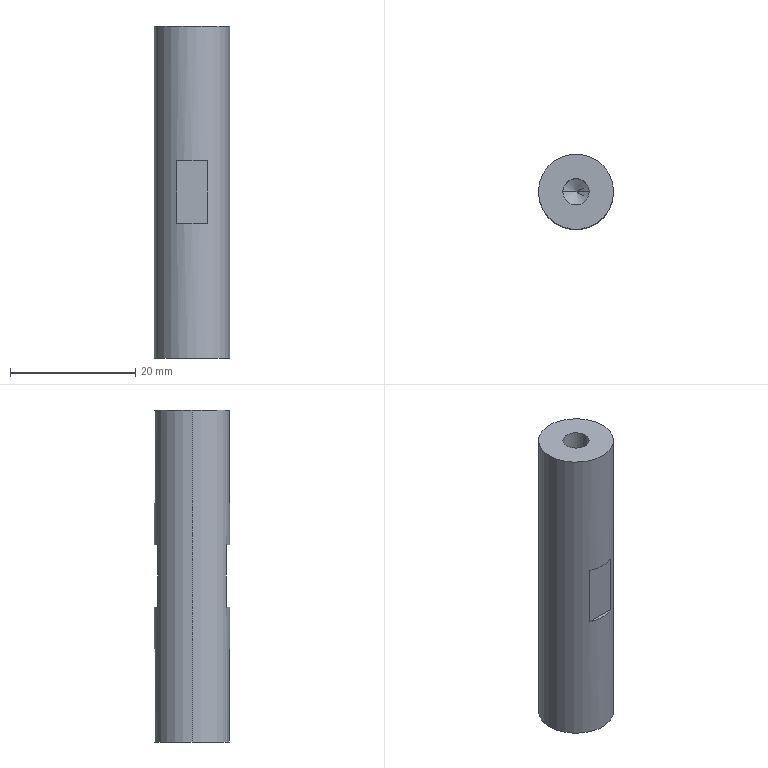Part | STEP file | 11-FG-E03911 | 1 solid | 18 faces | box 12 x 12 x 53 mm | volume 5607 mm3 | plane 8 | cylinder 6 | cone 4 | commonest cylinder face diameters 4.2 x4 12 x2
STEP:
#1=CARTESIAN_POINT('',(2.1,0.,12.4));
#2=VERTEX_POINT('',#1);
#3=CARTESIAN_POINT('',(-2.1,0.,12.4));
#4=VERTEX_POINT('',#3);
#5=CARTESIAN_POINT('',(0.,0.,12.4));
#6=DIRECTION('',(0.,0.,-1.));
#7=DIRECTION('',(-1.,0.,0.));
#8=AXIS2_PLACEMENT_3D('',#5,#6,#7);
#9=CIRCLE('',#8,2.1);
#10=EDGE_CURVE('',#2,#4,#9,.T.);
#11=ORIENTED_EDGE('',*,*,#10,.F.);
#12=CARTESIAN_POINT('',(2.1,0.,0.));
#13=VERTEX_POINT('',#12);
#14=CARTESIAN_POINT('',(2.1,0.,0.));
#15=DIRECTION('',(0.,0.,-1.));
#16=VECTOR('',#15,1000.);
#17=LINE('',#14,#16);
#18=EDGE_CURVE('',#2,#13,#17,.T.);
#19=ORIENTED_EDGE('',*,*,#18,.T.);
#20=CARTESIAN_POINT('',(-2.1,0.,0.));
#21=VERTEX_POINT('',#20);
#22=CARTESIAN_POINT('',(0.,0.,0.));
#23=DIRECTION('',(0.,0.,-1.));
#24=DIRECTION('',(-1.,0.,0.));
#25=AXIS2_PLACEMENT_3D('',#22,#23,#24);
#26=CIRCLE('',#25,2.1);
#27=EDGE_CURVE('',#13,#21,#26,.T.);
#28=ORIENTED_EDGE('',*,*,#27,.T.);
#29=CARTESIAN_POINT('',(-2.1,0.,0.));
#30=DIRECTION('',(0.,0.,-1.));
#31=VECTOR('',#30,1000.);
#32=LINE('',#29,#31);
#33=EDGE_CURVE('',#4,#21,#32,.T.);
#34=ORIENTED_EDGE('',*,*,#33,.F.);
#35=EDGE_LOOP('',(#11,#19,#28,#34));
#36=FACE_OUTER_BOUND('',#35,.T.);
#37=CARTESIAN_POINT('',(0.,0.,0.));
#38=DIRECTION('',(0.,0.,-1.));
#39=DIRECTION('',(-1.,0.,0.));
#40=AXIS2_PLACEMENT_3D('',#37,#38,#39);
#41=CYLINDRICAL_SURFACE('',#40,2.1);
#42=ADVANCED_FACE('',(#36),#41,.F.);
#43=CARTESIAN_POINT('',(0.,0.,13.662));
#44=VERTEX_POINT('',#43);
#45=CARTESIAN_POINT('',(-2.1,0.,12.4));
#46=DIRECTION('',(-0.8572,0.,-0.515));
#47=VECTOR('',#46,1000.);
#48=LINE('',#45,#47);
#49=EDGE_CURVE('',#44,#4,#48,.T.);
#50=ORIENTED_EDGE('',*,*,#49,.F.);
#51=CARTESIAN_POINT('',(2.1,0.,12.4));
#52=DIRECTION('',(0.8572,0.,-0.515));
#53=VECTOR('',#52,1000.);
#54=LINE('',#51,#53);
#55=EDGE_CURVE('',#44,#2,#54,.T.);
#56=ORIENTED_EDGE('',*,*,#55,.T.);
#57=ORIENTED_EDGE('',*,*,#10,.T.);
#58=EDGE_LOOP('',(#50,#56,#57));
#59=FACE_OUTER_BOUND('',#58,.T.);
#60=CARTESIAN_POINT('',(0.,0.,12.4));
#61=DIRECTION('',(0.,0.,-1.));
#62=DIRECTION('',(-1.,0.,0.));
#63=AXIS2_PLACEMENT_3D('',#60,#61,#62);
#64=CONICAL_SURFACE('',#63,2.1,1.03);
#65=ADVANCED_FACE('',(#59),#64,.F.);
#66=CARTESIAN_POINT('',(-2.1,0.,40.6));
#67=VERTEX_POINT('',#66);
#68=CARTESIAN_POINT('',(2.1,0.,40.6));
#69=VERTEX_POINT('',#68);
#70=CARTESIAN_POINT('',(0.,0.,40.6));
#71=DIRECTION('',(0.,0.,1.));
#72=DIRECTION('',(1.,0.,0.));
#73=AXIS2_PLACEMENT_3D('',#70,#71,#72);
#74=CIRCLE('',#73,2.1);
#75=EDGE_CURVE('',#67,#69,#74,.T.);
#76=ORIENTED_EDGE('',*,*,#75,.F.);
#77=CARTESIAN_POINT('',(-2.1,0.,53.));
#78=VERTEX_POINT('',#77);
#79=CARTESIAN_POINT('',(-2.1,0.,53.));
#80=DIRECTION('',(0.,0.,1.));
#81=VECTOR('',#80,1000.);
#82=LINE('',#79,#81);
#83=EDGE_CURVE('',#67,#78,#82,.T.);
#84=ORIENTED_EDGE('',*,*,#83,.T.);
#85=CARTESIAN_POINT('',(2.1,0.,53.));
#86=VERTEX_POINT('',#85);
#87=CARTESIAN_POINT('',(0.,0.,53.));
#88=DIRECTION('',(0.,0.,1.));
#89=DIRECTION('',(1.,0.,0.));
#90=AXIS2_PLACEMENT_3D('',#87,#88,#89);
#91=CIRCLE('',#90,2.1);
#92=EDGE_CURVE('',#78,#86,#91,.T.);
#93=ORIENTED_EDGE('',*,*,#92,.T.);
#94=CARTESIAN_POINT('',(2.1,0.,53.));
#95=DIRECTION('',(0.,0.,1.));
#96=VECTOR('',#95,1000.);
#97=LINE('',#94,#96);
#98=EDGE_CURVE('',#69,#86,#97,.T.);
#99=ORIENTED_EDGE('',*,*,#98,.F.);
#100=EDGE_LOOP('',(#76,#84,#93,#99));
#101=FACE_OUTER_BOUND('',#100,.T.);
#102=CARTESIAN_POINT('',(0.,0.,53.));
#103=DIRECTION('',(0.,0.,1.));
#104=DIRECTION('',(1.,0.,0.));
#105=AXIS2_PLACEMENT_3D('',#102,#103,#104);
#106=CYLINDRICAL_SURFACE('',#105,2.1);
#107=ADVANCED_FACE('',(#101),#106,.F.);
#108=CARTESIAN_POINT('',(0.,0.,39.338));
#109=VERTEX_POINT('',#108);
#110=CARTESIAN_POINT('',(2.1,0.,40.6));
#111=DIRECTION('',(0.8572,0.,0.515));
#112=VECTOR('',#111,1000.);
#113=LINE('',#110,#112);
#114=EDGE_CURVE('',#109,#69,#113,.T.);
#115=ORIENTED_EDGE('',*,*,#114,.F.);
#116=CARTESIAN_POINT('',(-2.1,0.,40.6));
#117=DIRECTION('',(-0.8572,0.,0.515));
#118=VECTOR('',#117,1000.);
#119=LINE('',#116,#118);
#120=EDGE_CURVE('',#109,#67,#119,.T.);
#121=ORIENTED_EDGE('',*,*,#120,.T.);
#122=ORIENTED_EDGE('',*,*,#75,.T.);
#123=EDGE_LOOP('',(#115,#121,#122));
#124=FACE_OUTER_BOUND('',#123,.T.);
#125=CARTESIAN_POINT('',(0.,0.,40.6));
#126=DIRECTION('',(0.,0.,1.));
#127=DIRECTION('',(1.,0.,0.));
#128=AXIS2_PLACEMENT_3D('',#125,#126,#127);
#129=CONICAL_SURFACE('',#128,2.1,1.03);
#130=ADVANCED_FACE('',(#124),#129,.F.);
#131=CARTESIAN_POINT('',(2.398,5.5,21.5));
#132=VERTEX_POINT('',#131);
#133=CARTESIAN_POINT('',(-2.398,5.5,21.5));
#134=VERTEX_POINT('',#133);
#135=CARTESIAN_POINT('',(0.,0.,21.5));
#136=DIRECTION('',(0.,0.,1.));
#137=DIRECTION('',(1.,0.,0.));
#138=AXIS2_PLACEMENT_3D('',#135,#136,#137);
#139=CIRCLE('',#138,6.);
#140=EDGE_CURVE('',#132,#134,#139,.T.);
#141=ORIENTED_EDGE('',*,*,#140,.F.);
#142=CARTESIAN_POINT('',(2.398,5.5,31.5));
#143=VERTEX_POINT('',#142);
#144=CARTESIAN_POINT('',(2.398,5.5,21.5));
#145=DIRECTION('',(0.,0.,1.));
#146=VECTOR('',#145,1000.);
#147=LINE('',#144,#146);
#148=EDGE_CURVE('',#132,#143,#147,.T.);
#149=ORIENTED_EDGE('',*,*,#148,.T.);
#150=CARTESIAN_POINT('',(-2.398,5.5,31.5));
#151=VERTEX_POINT('',#150);
#152=CARTESIAN_POINT('',(0.,0.,31.5));
#153=DIRECTION('',(0.,0.,1.));
#154=DIRECTION('',(1.,0.,0.));
#155=AXIS2_PLACEMENT_3D('',#152,#153,#154);
#156=CIRCLE('',#155,6.);
#157=EDGE_CURVE('',#143,#151,#156,.T.);
#158=ORIENTED_EDGE('',*,*,#157,.T.);
#159=CARTESIAN_POINT('',(-2.398,5.5,21.5));
#160=DIRECTION('',(0.,0.,1.));
#161=VECTOR('',#160,1000.);
#162=LINE('',#159,#161);
#163=EDGE_CURVE('',#134,#151,#162,.T.);
#164=ORIENTED_EDGE('',*,*,#163,.F.);
#165=EDGE_LOOP('',(#141,#149,#158,#164));
#166=FACE_BOUND('',#165,.T.);
#167=CARTESIAN_POINT('',(6.,0.,53.));
#168=VERTEX_POINT('',#167);
#169=CARTESIAN_POINT('',(-6.,0.,53.));
#170=VERTEX_POINT('',#169);
#171=CARTESIAN_POINT('',(0.,0.,53.));
#172=DIRECTION('',(0.,0.,1.));
#173=DIRECTION('',(1.,0.,0.));
#174=AXIS2_PLACEMENT_3D('',#171,#172,#173);
#175=CIRCLE('',#174,6.);
#176=EDGE_CURVE('',#168,#170,#175,.T.);
#177=ORIENTED_EDGE('',*,*,#176,.F.);
#178=CARTESIAN_POINT('',(6.,0.,0.));
#179=VERTEX_POINT('',#178);
#180=CARTESIAN_POINT('',(6.,0.,53.));
#181=DIRECTION('',(0.,0.,-1.));
#182=VECTOR('',#181,1000.);
#183=LINE('',#180,#182);
#184=EDGE_CURVE('',#168,#179,#183,.T.);
#185=ORIENTED_EDGE('',*,*,#184,.T.);
#186=CARTESIAN_POINT('',(-6.,0.,0.));
#187=VERTEX_POINT('',#186);
#188=CARTESIAN_POINT('',(0.,0.,0.));
#189=DIRECTION('',(0.,0.,1.));
#190=DIRECTION('',(1.,0.,0.));
#191=AXIS2_PLACEMENT_3D('',#188,#189,#190);
#192=CIRCLE('',#191,6.);
#193=EDGE_CURVE('',#179,#187,#192,.T.);
#194=ORIENTED_EDGE('',*,*,#193,.T.);
#195=CARTESIAN_POINT('',(-6.,0.,53.));
#196=DIRECTION('',(0.,0.,-1.));
#197=VECTOR('',#196,1000.);
#198=LINE('',#195,#197);
#199=EDGE_CURVE('',#170,#187,#198,.T.);
#200=ORIENTED_EDGE('',*,*,#199,.F.);
#201=EDGE_LOOP('',(#177,#185,#194,#200));
#202=FACE_OUTER_BOUND('',#201,.T.);
#203=CARTESIAN_POINT('',(0.,0.,53.));
#204=DIRECTION('',(0.,0.,-1.));
#205=DIRECTION('',(-1.,0.,0.));
#206=AXIS2_PLACEMENT_3D('',#203,#204,#205);
#207=CYLINDRICAL_SURFACE('',#206,6.);
#208=ADVANCED_FACE('',(#166,#202),#207,.T.);
#209=ORIENTED_EDGE('',*,*,#184,.F.);
#210=CARTESIAN_POINT('',(0.,0.,53.));
#211=DIRECTION('',(0.,0.,1.));
#212=DIRECTION('',(1.,0.,0.));
#213=AXIS2_PLACEMENT_3D('',#210,#211,#212);
#214=CIRCLE('',#213,6.);
#215=EDGE_CURVE('',#170,#168,#214,.T.);
#216=ORIENTED_EDGE('',*,*,#215,.F.);
#217=ORIENTED_EDGE('',*,*,#199,.T.);
#218=CARTESIAN_POINT('',(0.,0.,0.));
#219=DIRECTION('',(0.,0.,1.));
#220=DIRECTION('',(1.,0.,0.));
#221=AXIS2_PLACEMENT_3D('',#218,#219,#220);
#222=CIRCLE('',#221,6.);
#223=EDGE_CURVE('',#187,#179,#222,.T.);
#224=ORIENTED_EDGE('',*,*,#223,.T.);
#225=EDGE_LOOP('',(#209,#216,#217,#224));
#226=FACE_OUTER_BOUND('',#225,.T.);
#227=CARTESIAN_POINT('',(-2.398,-5.5,21.5));
#228=VERTEX_POINT('',#227);
#229=CARTESIAN_POINT('',(2.398,-5.5,21.5));
#230=VERTEX_POINT('',#229);
#231=CARTESIAN_POINT('',(0.,0.,21.5));
#232=DIRECTION('',(0.,0.,1.));
#233=DIRECTION('',(1.,0.,0.));
#234=AXIS2_PLACEMENT_3D('',#231,#232,#233);
#235=CIRCLE('',#234,6.);
#236=EDGE_CURVE('',#228,#230,#235,.T.);
#237=ORIENTED_EDGE('',*,*,#236,.F.);
#238=CARTESIAN_POINT('',(-2.398,-5.5,31.5));
#239=VERTEX_POINT('',#238);
#240=CARTESIAN_POINT('',(-2.398,-5.5,21.5));
#241=DIRECTION('',(0.,0.,1.));
#242=VECTOR('',#241,1000.);
#243=LINE('',#240,#242);
#244=EDGE_CURVE('',#228,#239,#243,.T.);
#245=ORIENTED_EDGE('',*,*,#244,.T.);
#246=CARTESIAN_POINT('',(2.398,-5.5,31.5));
#247=VERTEX_POINT('',#246);
#248=CARTESIAN_POINT('',(0.,0.,31.5));
#249=DIRECTION('',(0.,0.,1.));
#250=DIRECTION('',(1.,0.,0.));
#251=AXIS2_PLACEMENT_3D('',#248,#249,#250);
#252=CIRCLE('',#251,6.);
#253=EDGE_CURVE('',#239,#247,#252,.T.);
#254=ORIENTED_EDGE('',*,*,#253,.T.);
#255=CARTESIAN_POINT('',(2.398,-5.5,21.5));
#256=DIRECTION('',(0.,0.,1.));
#257=VECTOR('',#256,1000.);
#258=LINE('',#255,#257);
#259=EDGE_CURVE('',#230,#247,#258,.T.);
#260=ORIENTED_EDGE('',*,*,#259,.F.);
#261=EDGE_LOOP('',(#237,#245,#254,#260));
#262=FACE_BOUND('',#261,.T.);
#263=CARTESIAN_POINT('',(0.,0.,53.));
#264=DIRECTION('',(0.,0.,-1.));
#265=DIRECTION('',(-1.,0.,0.));
#266=AXIS2_PLACEMENT_3D('',#263,#264,#265);
#267=CYLINDRICAL_SURFACE('',#266,6.);
#268=ADVANCED_FACE('',(#226,#262),#267,.T.);
#269=CARTESIAN_POINT('',(0.,0.,53.));
#270=DIRECTION('',(0.,0.,1.));
#271=DIRECTION('',(1.,0.,0.));
#272=AXIS2_PLACEMENT_3D('',#269,#270,#271);
#273=CIRCLE('',#272,2.1);
#274=EDGE_CURVE('',#86,#78,#273,.T.);
#275=ORIENTED_EDGE('',*,*,#274,.F.);
#276=ORIENTED_EDGE('',*,*,#92,.F.);
#277=EDGE_LOOP('',(#275,#276));
#278=FACE_BOUND('',#277,.T.);
#279=ORIENTED_EDGE('',*,*,#215,.T.);
#280=ORIENTED_EDGE('',*,*,#176,.T.);
#281=EDGE_LOOP('',(#279,#280));
#282=FACE_OUTER_BOUND('',#281,.T.);
#283=CARTESIAN_POINT('',(0.,0.,53.));
#284=DIRECTION('',(0.,0.,1.));
#285=DIRECTION('',(1.,0.,0.));
#286=AXIS2_PLACEMENT_3D('',#283,#284,#285);
#287=PLANE('',#286);
#288=ADVANCED_FACE('',(#278,#282),#287,.T.);
#289=CARTESIAN_POINT('',(0.,0.,0.));
#290=DIRECTION('',(0.,0.,-1.));
#291=DIRECTION('',(-1.,0.,0.));
#292=AXIS2_PLACEMENT_3D('',#289,#290,#291);
#293=CIRCLE('',#292,2.1);
#294=EDGE_CURVE('',#21,#13,#293,.T.);
#295=ORIENTED_EDGE('',*,*,#294,.F.);
#296=ORIENTED_EDGE('',*,*,#27,.F.);
#297=EDGE_LOOP('',(#295,#296));
#298=FACE_BOUND('',#297,.T.);
#299=ORIENTED_EDGE('',*,*,#223,.F.);
#300=ORIENTED_EDGE('',*,*,#193,.F.);
#301=EDGE_LOOP('',(#299,#300));
#302=FACE_OUTER_BOUND('',#301,.T.);
#303=CARTESIAN_POINT('',(0.,0.,0.));
#304=DIRECTION('',(0.,0.,1.));
#305=DIRECTION('',(1.,0.,0.));
#306=AXIS2_PLACEMENT_3D('',#303,#304,#305);
#307=PLANE('',#306);
#308=ADVANCED_FACE('',(#298,#302),#307,.F.);
#309=ORIENTED_EDGE('',*,*,#120,.F.);
#310=ORIENTED_EDGE('',*,*,#114,.T.);
#311=CARTESIAN_POINT('',(0.,0.,40.6));
#312=DIRECTION('',(0.,0.,1.));
#313=DIRECTION('',(1.,0.,0.));
#314=AXIS2_PLACEMENT_3D('',#311,#312,#313);
#315=CIRCLE('',#314,2.1);
#316=EDGE_CURVE('',#69,#67,#315,.T.);
#317=ORIENTED_EDGE('',*,*,#316,.T.);
#318=EDGE_LOOP('',(#309,#310,#317));
#319=FACE_OUTER_BOUND('',#318,.T.);
#320=CARTESIAN_POINT('',(0.,0.,40.6));
#321=DIRECTION('',(0.,0.,1.));
#322=DIRECTION('',(1.,0.,0.));
#323=AXIS2_PLACEMENT_3D('',#320,#321,#322);
#324=CONICAL_SURFACE('',#323,2.1,1.03);
#325=ADVANCED_FACE('',(#319),#324,.F.);
#326=ORIENTED_EDGE('',*,*,#83,.F.);
#327=ORIENTED_EDGE('',*,*,#316,.F.);
#328=ORIENTED_EDGE('',*,*,#98,.T.);
#329=ORIENTED_EDGE('',*,*,#274,.T.);
#330=EDGE_LOOP('',(#326,#327,#328,#329));
#331=FACE_OUTER_BOUND('',#330,.T.);
#332=CARTESIAN_POINT('',(0.,0.,53.));
#333=DIRECTION('',(0.,0.,1.));
#334=DIRECTION('',(1.,0.,0.));
#335=AXIS2_PLACEMENT_3D('',#332,#333,#334);
#336=CYLINDRICAL_SURFACE('',#335,2.1);
#337=ADVANCED_FACE('',(#331),#336,.F.);
#338=ORIENTED_EDGE('',*,*,#55,.F.);
#339=ORIENTED_EDGE('',*,*,#49,.T.);
#340=CARTESIAN_POINT('',(0.,0.,12.4));
#341=DIRECTION('',(0.,0.,-1.));
#342=DIRECTION('',(-1.,0.,0.));
#343=AXIS2_PLACEMENT_3D('',#340,#341,#342);
#344=CIRCLE('',#343,2.1);
#345=EDGE_CURVE('',#4,#2,#344,.T.);
#346=ORIENTED_EDGE('',*,*,#345,.T.);
#347=EDGE_LOOP('',(#338,#339,#346));
#348=FACE_OUTER_BOUND('',#347,.T.);
#349=CARTESIAN_POINT('',(0.,0.,12.4));
#350=DIRECTION('',(0.,0.,-1.));
#351=DIRECTION('',(-1.,0.,0.));
#352=AXIS2_PLACEMENT_3D('',#349,#350,#351);
#353=CONICAL_SURFACE('',#352,2.1,1.03);
#354=ADVANCED_FACE('',(#348),#353,.F.);
#355=ORIENTED_EDGE('',*,*,#18,.F.);
#356=ORIENTED_EDGE('',*,*,#345,.F.);
#357=ORIENTED_EDGE('',*,*,#33,.T.);
#358=ORIENTED_EDGE('',*,*,#294,.T.);
#359=EDGE_LOOP('',(#355,#356,#357,#358));
#360=FACE_OUTER_BOUND('',#359,.T.);
#361=CARTESIAN_POINT('',(0.,0.,0.));
#362=DIRECTION('',(0.,0.,-1.));
#363=DIRECTION('',(-1.,0.,0.));
#364=AXIS2_PLACEMENT_3D('',#361,#362,#363);
#365=CYLINDRICAL_SURFACE('',#364,2.1);
#366=ADVANCED_FACE('',(#360),#365,.F.);
#367=CARTESIAN_POINT('',(-2.398,5.5,31.5));
#368=DIRECTION('',(1.,0.,0.));
#369=VECTOR('',#368,1000.);
#370=LINE('',#367,#369);
#371=EDGE_CURVE('',#151,#143,#370,.T.);
#372=ORIENTED_EDGE('',*,*,#371,.T.);
#373=ORIENTED_EDGE('',*,*,#148,.F.);
#374=CARTESIAN_POINT('',(-2.398,5.5,21.5));
#375=DIRECTION('',(1.,0.,0.));
#376=VECTOR('',#375,1000.);
#377=LINE('',#374,#376);
#378=EDGE_CURVE('',#134,#132,#377,.T.);
#379=ORIENTED_EDGE('',*,*,#378,.F.);
#380=ORIENTED_EDGE('',*,*,#163,.T.);
#381=EDGE_LOOP('',(#372,#373,#379,#380));
#382=FACE_OUTER_BOUND('',#381,.T.);
#383=CARTESIAN_POINT('',(-2.398,5.5,21.5));
#384=DIRECTION('',(0.,-1.,0.));
#385=DIRECTION('',(0.,0.,-1.));
#386=AXIS2_PLACEMENT_3D('',#383,#384,#385);
#387=PLANE('',#386);
#388=ADVANCED_FACE('',(#382),#387,.F.);
#389=ORIENTED_EDGE('',*,*,#140,.T.);
#390=ORIENTED_EDGE('',*,*,#378,.T.);
#391=EDGE_LOOP('',(#389,#390));
#392=FACE_OUTER_BOUND('',#391,.T.);
#393=CARTESIAN_POINT('',(0.,0.,21.5));
#394=DIRECTION('',(0.,0.,1.));
#395=DIRECTION('',(1.,0.,0.));
#396=AXIS2_PLACEMENT_3D('',#393,#394,#395);
#397=PLANE('',#396);
#398=ADVANCED_FACE('',(#392),#397,.T.);
#399=ORIENTED_EDGE('',*,*,#157,.F.);
#400=ORIENTED_EDGE('',*,*,#371,.F.);
#401=EDGE_LOOP('',(#399,#400));
#402=FACE_OUTER_BOUND('',#401,.T.);
#403=CARTESIAN_POINT('',(0.,0.,31.5));
#404=DIRECTION('',(0.,0.,1.));
#405=DIRECTION('',(1.,0.,0.));
#406=AXIS2_PLACEMENT_3D('',#403,#404,#405);
#407=PLANE('',#406);
#408=ADVANCED_FACE('',(#402),#407,.F.);
#409=CARTESIAN_POINT('',(-2.398,-5.5,31.5));
#410=DIRECTION('',(-1.,0.,0.));
#411=VECTOR('',#410,1000.);
#412=LINE('',#409,#411);
#413=EDGE_CURVE('',#247,#239,#412,.T.);
#414=ORIENTED_EDGE('',*,*,#413,.T.);
#415=ORIENTED_EDGE('',*,*,#244,.F.);
#416=CARTESIAN_POINT('',(-2.398,-5.5,21.5));
#417=DIRECTION('',(-1.,0.,0.));
#418=VECTOR('',#417,1000.);
#419=LINE('',#416,#418);
#420=EDGE_CURVE('',#230,#228,#419,.T.);
#421=ORIENTED_EDGE('',*,*,#420,.F.);
#422=ORIENTED_EDGE('',*,*,#259,.T.);
#423=EDGE_LOOP('',(#414,#415,#421,#422));
#424=FACE_OUTER_BOUND('',#423,.T.);
#425=CARTESIAN_POINT('',(-2.398,-5.5,21.5));
#426=DIRECTION('',(0.,1.,0.));
#427=DIRECTION('',(0.,0.,1.));
#428=AXIS2_PLACEMENT_3D('',#425,#426,#427);
#429=PLANE('',#428);
#430=ADVANCED_FACE('',(#424),#429,.F.);
#431=ORIENTED_EDGE('',*,*,#236,.T.);
#432=ORIENTED_EDGE('',*,*,#420,.T.);
#433=EDGE_LOOP('',(#431,#432));
#434=FACE_OUTER_BOUND('',#433,.T.);
#435=CARTESIAN_POINT('',(0.,0.,21.5));
#436=DIRECTION('',(0.,0.,1.));
#437=DIRECTION('',(1.,0.,0.));
#438=AXIS2_PLACEMENT_3D('',#435,#436,#437);
#439=PLANE('',#438);
#440=ADVANCED_FACE('',(#434),#439,.T.);
#441=ORIENTED_EDGE('',*,*,#253,.F.);
#442=ORIENTED_EDGE('',*,*,#413,.F.);
#443=EDGE_LOOP('',(#441,#442));
#444=FACE_OUTER_BOUND('',#443,.T.);
#445=CARTESIAN_POINT('',(0.,0.,31.5));
#446=DIRECTION('',(0.,0.,1.));
#447=DIRECTION('',(1.,0.,0.));
#448=AXIS2_PLACEMENT_3D('',#445,#446,#447);
#449=PLANE('',#448);
#450=ADVANCED_FACE('',(#444),#449,.F.);
#451=CLOSED_SHELL('',(#42,#65,#107,#130,#208,#268,#288,#308,#325,#337,#354,#366,#388,#398,#408,#430,#440,#450));
#452=MANIFOLD_SOLID_BREP('',#451);
#453=CARTESIAN_POINT('',(0.,0.,0.));
#454=DIRECTION('',(0.,0.,1.));
#455=DIRECTION('',(1.,0.,0.));
#456=AXIS2_PLACEMENT_3D('',#453,#454,#455);
#457=(LENGTH_UNIT()NAMED_UNIT(*)SI_UNIT(.MILLI.,.METRE.));
#458=UNCERTAINTY_MEASURE_WITH_UNIT(LENGTH_MEASURE(0.00001),#457,'','');
#459=(NAMED_UNIT(*)PLANE_ANGLE_UNIT()SI_UNIT($,.RADIAN.));
#460=(NAMED_UNIT(*)SI_UNIT($,.STERADIAN.)SOLID_ANGLE_UNIT());
#461=(GEOMETRIC_REPRESENTATION_CONTEXT(3)GLOBAL_UNCERTAINTY_ASSIGNED_CONTEXT((#458))GLOBAL_UNIT_ASSIGNED_CONTEXT((#457,#459,#460))REPRESENTATION_CONTEXT('',''));
#462=ADVANCED_BREP_SHAPE_REPRESENTATION('',(#452,#456),#461);